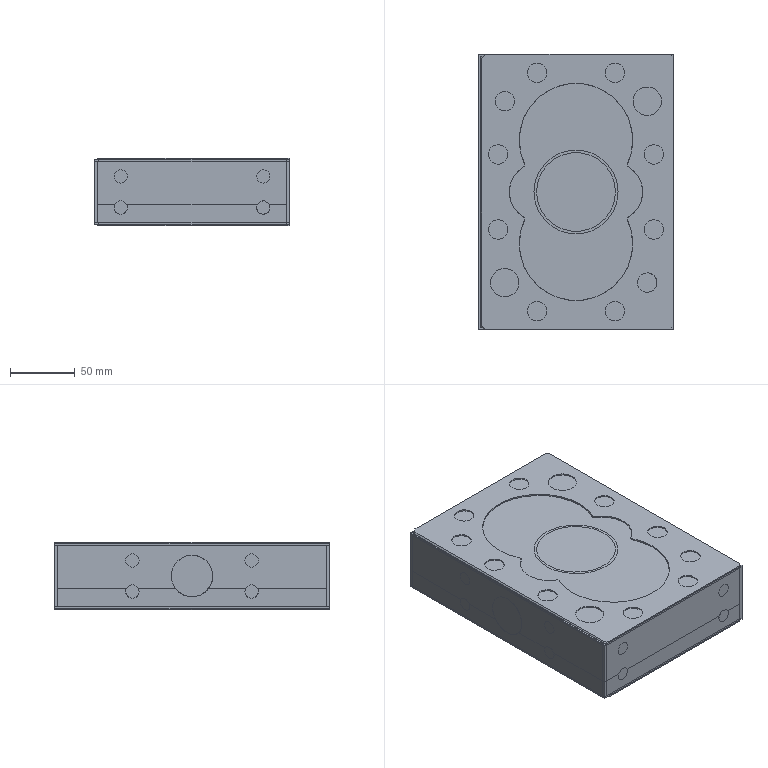NC program | NX | posted with a generic post | part box 150.2 x 212.2 x 52.4 mm
Lines 1 to 17 of 152230:
N10 G17 G21 G94 G90
(G81点孔_6 , TOOL : Z3.3钻头)
N12 T04 M6
N14 /M1
N16 G54
N18 G17 G0 G90 X0. Y0. S300 M3
N20 G43 Z100. H4
N22 G94 G81 G98 Z-52. F10. R1.5
N24 X-40.
N26 X40.
N28 G80
N30 G0 X40. Y0. Z100.
N32 M5